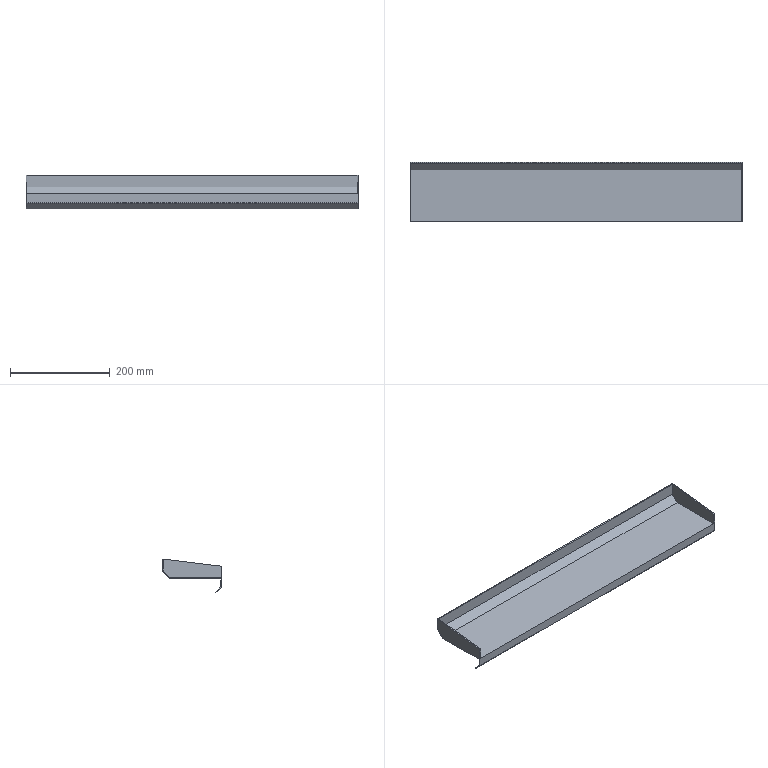Part | SolidWorks | features ICE 2, Chamfer 1, Extrusion 1, Shell 1 | 1 solid | 18 faces | box 665 x 120 x 68.021 mm | volume 255625 mm3 | plane 16 | cylinder 2 | commonest cylinder face diameters 4 x2
STEP:
#1=CARTESIAN_POINT('',(-332.5,-118.,-40.));
#2=VERTEX_POINT('',#1);
#3=CARTESIAN_POINT('',(332.5,-118.,-40.));
#4=VERTEX_POINT('',#3);
#5=CARTESIAN_POINT('',(-363.575,-118.,-40.));
#6=DIRECTION('',(1.,0.,0.));
#7=VECTOR('',#6,1000.);
#8=LINE('',#5,#7);
#9=EDGE_CURVE('',#2,#4,#8,.T.);
#10=ORIENTED_EDGE('',*,*,#9,.F.);
#11=CARTESIAN_POINT('',(-332.5,-15.,-40.));
#12=VERTEX_POINT('',#11);
#13=CARTESIAN_POINT('',(-332.5,0.,-40.));
#14=DIRECTION('',(0.,1.,0.));
#15=VECTOR('',#14,1000.);
#16=LINE('',#13,#15);
#17=EDGE_CURVE('',#2,#12,#16,.T.);
#18=ORIENTED_EDGE('',*,*,#17,.T.);
#19=CARTESIAN_POINT('',(332.5,-15.,-40.));
#20=VERTEX_POINT('',#19);
#21=CARTESIAN_POINT('',(332.5,-15.,-40.));
#22=DIRECTION('',(1.,0.,0.));
#23=VECTOR('',#22,1000.);
#24=LINE('',#21,#23);
#25=EDGE_CURVE('',#12,#20,#24,.T.);
#26=ORIENTED_EDGE('',*,*,#25,.T.);
#27=CARTESIAN_POINT('',(332.5,0.,-40.));
#28=DIRECTION('',(0.,1.,0.));
#29=VECTOR('',#28,1000.);
#30=LINE('',#27,#29);
#31=EDGE_CURVE('',#4,#20,#30,.T.);
#32=ORIENTED_EDGE('',*,*,#31,.F.);
#33=EDGE_LOOP('',(#10,#18,#26,#32));
#34=FACE_OUTER_BOUND('',#33,.T.);
#35=CARTESIAN_POINT('',(332.5,0.,-40.));
#36=DIRECTION('',(0.,0.,1.));
#37=DIRECTION('',(0.,-1.,0.));
#38=AXIS2_PLACEMENT_3D('',#35,#36,#37);
#39=PLANE('',#38);
#40=ADVANCED_FACE('',(#34),#39,.F.);
#41=CARTESIAN_POINT('',(330.5,-2.,-0.2408));
#42=VERTEX_POINT('',#41);
#43=CARTESIAN_POINT('',(330.5,-120.,-14.447));
#44=VERTEX_POINT('',#43);
#45=CARTESIAN_POINT('',(330.5,0.,0.));
#46=DIRECTION('',(0.,-0.9928,-0.1195));
#47=VECTOR('',#46,1000.);
#48=LINE('',#45,#47);
#49=EDGE_CURVE('',#42,#44,#48,.T.);
#50=ORIENTED_EDGE('',*,*,#49,.T.);
#51=CARTESIAN_POINT('',(332.5,-120.,-14.447));
#52=VERTEX_POINT('',#51);
#53=CARTESIAN_POINT('',(332.5,-120.,-14.447));
#54=DIRECTION('',(-1.,0.,0.));
#55=VECTOR('',#54,1000.);
#56=LINE('',#53,#55);
#57=EDGE_CURVE('',#52,#44,#56,.T.);
#58=ORIENTED_EDGE('',*,*,#57,.F.);
#59=CARTESIAN_POINT('',(332.5,0.,0.));
#60=VERTEX_POINT('',#59);
#61=CARTESIAN_POINT('',(332.5,-120.,-14.447));
#62=DIRECTION('',(0.,-0.9928,-0.1195));
#63=VECTOR('',#62,1000.);
#64=LINE('',#61,#63);
#65=EDGE_CURVE('',#60,#52,#64,.T.);
#66=ORIENTED_EDGE('',*,*,#65,.F.);
#67=CARTESIAN_POINT('',(-332.5,0.,0.));
#68=VERTEX_POINT('',#67);
#69=CARTESIAN_POINT('',(332.5,0.,0.));
#70=DIRECTION('',(-1.,0.,0.));
#71=VECTOR('',#70,1000.);
#72=LINE('',#69,#71);
#73=EDGE_CURVE('',#60,#68,#72,.T.);
#74=ORIENTED_EDGE('',*,*,#73,.T.);
#75=CARTESIAN_POINT('',(-332.5,-120.,-14.447));
#76=VERTEX_POINT('',#75);
#77=CARTESIAN_POINT('',(-332.5,-120.,-14.447));
#78=DIRECTION('',(0.,-0.9928,-0.1195));
#79=VECTOR('',#78,1000.);
#80=LINE('',#77,#79);
#81=EDGE_CURVE('',#68,#76,#80,.T.);
#82=ORIENTED_EDGE('',*,*,#81,.T.);
#83=CARTESIAN_POINT('',(-330.5,-120.,-14.447));
#84=VERTEX_POINT('',#83);
#85=CARTESIAN_POINT('',(332.5,-120.,-14.447));
#86=DIRECTION('',(-1.,0.,0.));
#87=VECTOR('',#86,1000.);
#88=LINE('',#85,#87);
#89=EDGE_CURVE('',#84,#76,#88,.T.);
#90=ORIENTED_EDGE('',*,*,#89,.F.);
#91=CARTESIAN_POINT('',(-330.5,-2.,-0.2408));
#92=VERTEX_POINT('',#91);
#93=CARTESIAN_POINT('',(-330.5,0.,0.));
#94=DIRECTION('',(0.,-0.9928,-0.1195));
#95=VECTOR('',#94,1000.);
#96=LINE('',#93,#95);
#97=EDGE_CURVE('',#92,#84,#96,.T.);
#98=ORIENTED_EDGE('',*,*,#97,.F.);
#99=CARTESIAN_POINT('',(332.5,-2.,-0.2408));
#100=DIRECTION('',(-1.,0.,0.));
#101=VECTOR('',#100,1000.);
#102=LINE('',#99,#101);
#103=EDGE_CURVE('',#42,#92,#102,.T.);
#104=ORIENTED_EDGE('',*,*,#103,.F.);
#105=EDGE_LOOP('',(#50,#58,#66,#74,#82,#90,#98,#104));
#106=FACE_OUTER_BOUND('',#105,.T.);
#107=CARTESIAN_POINT('',(332.5,-120.,-14.447));
#108=DIRECTION('',(0.,0.1195,-0.9928));
#109=DIRECTION('',(0.,0.9928,0.1195));
#110=AXIS2_PLACEMENT_3D('',#107,#108,#109);
#111=PLANE('',#110);
#112=ADVANCED_FACE('',(#106),#111,.F.);
#113=ORIENTED_EDGE('',*,*,#57,.T.);
#114=CARTESIAN_POINT('',(330.5,-120.,-38.));
#115=VERTEX_POINT('',#114);
#116=CARTESIAN_POINT('',(330.5,-120.,-14.206));
#117=DIRECTION('',(0.,0.,-1.));
#118=VECTOR('',#117,1000.);
#119=LINE('',#116,#118);
#120=EDGE_CURVE('',#44,#115,#119,.T.);
#121=ORIENTED_EDGE('',*,*,#120,.T.);
#122=CARTESIAN_POINT('',(-330.5,-120.,-38.));
#123=VERTEX_POINT('',#122);
#124=CARTESIAN_POINT('',(330.5,-120.,-38.));
#125=DIRECTION('',(-1.,0.,0.));
#126=VECTOR('',#125,1000.);
#127=LINE('',#124,#126);
#128=EDGE_CURVE('',#115,#123,#127,.T.);
#129=ORIENTED_EDGE('',*,*,#128,.T.);
#130=CARTESIAN_POINT('',(-330.5,-120.,-38.));
#131=DIRECTION('',(0.,0.,1.));
#132=VECTOR('',#131,1000.);
#133=LINE('',#130,#132);
#134=EDGE_CURVE('',#123,#84,#133,.T.);
#135=ORIENTED_EDGE('',*,*,#134,.T.);
#136=ORIENTED_EDGE('',*,*,#89,.T.);
#137=CARTESIAN_POINT('',(-332.5,-120.,-55.172));
#138=VERTEX_POINT('',#137);
#139=CARTESIAN_POINT('',(-332.5,-120.,-14.447));
#140=DIRECTION('',(0.,0.,-1.));
#141=VECTOR('',#140,1000.);
#142=LINE('',#139,#141);
#143=EDGE_CURVE('',#76,#138,#142,.T.);
#144=ORIENTED_EDGE('',*,*,#143,.T.);
#145=CARTESIAN_POINT('',(332.5,-120.,-55.172));
#146=VERTEX_POINT('',#145);
#147=CARTESIAN_POINT('',(-363.575,-120.,-55.172));
#148=DIRECTION('',(1.,0.,0.));
#149=VECTOR('',#148,1000.);
#150=LINE('',#147,#149);
#151=EDGE_CURVE('',#138,#146,#150,.T.);
#152=ORIENTED_EDGE('',*,*,#151,.T.);
#153=CARTESIAN_POINT('',(332.5,-120.,-14.447));
#154=DIRECTION('',(0.,0.,-1.));
#155=VECTOR('',#154,1000.);
#156=LINE('',#153,#155);
#157=EDGE_CURVE('',#52,#146,#156,.T.);
#158=ORIENTED_EDGE('',*,*,#157,.F.);
#159=EDGE_LOOP('',(#113,#121,#129,#135,#136,#144,#152,#158));
#160=FACE_OUTER_BOUND('',#159,.T.);
#161=CARTESIAN_POINT('',(332.5,-120.,-14.447));
#162=DIRECTION('',(0.,1.,0.));
#163=DIRECTION('',(0.,0.,1.));
#164=AXIS2_PLACEMENT_3D('',#161,#162,#163);
#165=PLANE('',#164);
#166=ADVANCED_FACE('',(#160),#165,.F.);
#167=CARTESIAN_POINT('',(332.5,0.,-25.));
#168=VERTEX_POINT('',#167);
#169=CARTESIAN_POINT('',(332.5,0.,0.));
#170=DIRECTION('',(0.,0.,1.));
#171=VECTOR('',#170,1000.);
#172=LINE('',#169,#171);
#173=EDGE_CURVE('',#168,#60,#172,.T.);
#174=ORIENTED_EDGE('',*,*,#173,.F.);
#175=CARTESIAN_POINT('',(-332.5,0.,-25.));
#176=VERTEX_POINT('',#175);
#177=CARTESIAN_POINT('',(332.5,0.,-25.));
#178=DIRECTION('',(-1.,0.,0.));
#179=VECTOR('',#178,1000.);
#180=LINE('',#177,#179);
#181=EDGE_CURVE('',#168,#176,#180,.T.);
#182=ORIENTED_EDGE('',*,*,#181,.T.);
#183=CARTESIAN_POINT('',(-332.5,0.,0.));
#184=DIRECTION('',(0.,0.,1.));
#185=VECTOR('',#184,1000.);
#186=LINE('',#183,#185);
#187=EDGE_CURVE('',#176,#68,#186,.T.);
#188=ORIENTED_EDGE('',*,*,#187,.T.);
#189=ORIENTED_EDGE('',*,*,#73,.F.);
#190=EDGE_LOOP('',(#174,#182,#188,#189));
#191=FACE_OUTER_BOUND('',#190,.T.);
#192=CARTESIAN_POINT('',(332.5,0.,0.));
#193=DIRECTION('',(0.,-1.,0.));
#194=DIRECTION('',(0.,0.,-1.));
#195=AXIS2_PLACEMENT_3D('',#192,#193,#194);
#196=PLANE('',#195);
#197=ADVANCED_FACE('',(#191),#196,.F.);
#198=ORIENTED_EDGE('',*,*,#157,.T.);
#199=CARTESIAN_POINT('',(332.5,-119.414,-56.586));
#200=VERTEX_POINT('',#199);
#201=CARTESIAN_POINT('',(332.5,-118.,-55.172));
#202=DIRECTION('',(1.,0.,0.));
#203=DIRECTION('',(0.,0.,1.));
#204=AXIS2_PLACEMENT_3D('',#201,#202,#203);
#205=CIRCLE('',#204,2.);
#206=EDGE_CURVE('',#146,#200,#205,.T.);
#207=ORIENTED_EDGE('',*,*,#206,.T.);
#208=CARTESIAN_POINT('',(332.5,-107.979,-68.021));
#209=VERTEX_POINT('',#208);
#210=CARTESIAN_POINT('',(332.5,-119.414,-56.586));
#211=DIRECTION('',(0.,0.7071,-0.7071));
#212=VECTOR('',#211,1000.);
#213=LINE('',#210,#212);
#214=EDGE_CURVE('',#200,#209,#213,.T.);
#215=ORIENTED_EDGE('',*,*,#214,.T.);
#216=CARTESIAN_POINT('',(332.5,-106.565,-66.607));
#217=VERTEX_POINT('',#216);
#218=CARTESIAN_POINT('',(332.5,-107.979,-68.021));
#219=DIRECTION('',(0.,0.7071,0.7071));
#220=VECTOR('',#219,1000.);
#221=LINE('',#218,#220);
#222=EDGE_CURVE('',#209,#217,#221,.T.);
#223=ORIENTED_EDGE('',*,*,#222,.T.);
#224=CARTESIAN_POINT('',(332.5,-117.414,-55.757));
#225=VERTEX_POINT('',#224);
#226=CARTESIAN_POINT('',(332.5,-106.565,-66.607));
#227=DIRECTION('',(0.,-0.7071,0.7071));
#228=VECTOR('',#227,1000.);
#229=LINE('',#226,#228);
#230=EDGE_CURVE('',#217,#225,#229,.T.);
#231=ORIENTED_EDGE('',*,*,#230,.T.);
#232=CARTESIAN_POINT('',(332.5,-118.,-54.343));
#233=VERTEX_POINT('',#232);
#234=CARTESIAN_POINT('',(332.5,-116.,-54.343));
#235=DIRECTION('',(-1.,0.,0.));
#236=DIRECTION('',(0.,0.,1.));
#237=AXIS2_PLACEMENT_3D('',#234,#235,#236);
#238=CIRCLE('',#237,2.);
#239=EDGE_CURVE('',#225,#233,#238,.T.);
#240=ORIENTED_EDGE('',*,*,#239,.T.);
#241=CARTESIAN_POINT('',(332.5,-118.,-54.343));
#242=DIRECTION('',(0.,0.,1.));
#243=VECTOR('',#242,1000.);
#244=LINE('',#241,#243);
#245=EDGE_CURVE('',#233,#4,#244,.T.);
#246=ORIENTED_EDGE('',*,*,#245,.T.);
#247=ORIENTED_EDGE('',*,*,#31,.T.);
#248=CARTESIAN_POINT('',(332.5,0.,-25.));
#249=DIRECTION('',(0.,0.7071,0.7071));
#250=VECTOR('',#249,1000.);
#251=LINE('',#248,#250);
#252=EDGE_CURVE('',#20,#168,#251,.T.);
#253=ORIENTED_EDGE('',*,*,#252,.T.);
#254=ORIENTED_EDGE('',*,*,#173,.T.);
#255=ORIENTED_EDGE('',*,*,#65,.T.);
#256=EDGE_LOOP('',(#198,#207,#215,#223,#231,#240,#246,#247,#253,#254,#255));
#257=FACE_OUTER_BOUND('',#256,.T.);
#258=CARTESIAN_POINT('',(332.5,0.,0.));
#259=DIRECTION('',(-1.,0.,0.));
#260=DIRECTION('',(0.,0.,1.));
#261=AXIS2_PLACEMENT_3D('',#258,#259,#260);
#262=PLANE('',#261);
#263=ADVANCED_FACE('',(#257),#262,.F.);
#264=ORIENTED_EDGE('',*,*,#187,.F.);
#265=CARTESIAN_POINT('',(-332.5,12.5,-12.5));
#266=DIRECTION('',(0.,-0.7071,-0.7071));
#267=VECTOR('',#266,1000.);
#268=LINE('',#265,#267);
#269=EDGE_CURVE('',#176,#12,#268,.T.);
#270=ORIENTED_EDGE('',*,*,#269,.T.);
#271=ORIENTED_EDGE('',*,*,#17,.F.);
#272=CARTESIAN_POINT('',(-332.5,-118.,-54.343));
#273=VERTEX_POINT('',#272);
#274=CARTESIAN_POINT('',(-332.5,-118.,-54.343));
#275=DIRECTION('',(0.,0.,1.));
#276=VECTOR('',#275,1000.);
#277=LINE('',#274,#276);
#278=EDGE_CURVE('',#273,#2,#277,.T.);
#279=ORIENTED_EDGE('',*,*,#278,.F.);
#280=CARTESIAN_POINT('',(-332.5,-117.414,-55.757));
#281=VERTEX_POINT('',#280);
#282=CARTESIAN_POINT('',(-332.5,-116.,-54.343));
#283=DIRECTION('',(-1.,0.,0.));
#284=DIRECTION('',(0.,0.,1.));
#285=AXIS2_PLACEMENT_3D('',#282,#283,#284);
#286=CIRCLE('',#285,2.);
#287=EDGE_CURVE('',#281,#273,#286,.T.);
#288=ORIENTED_EDGE('',*,*,#287,.F.);
#289=CARTESIAN_POINT('',(-332.5,-106.565,-66.607));
#290=VERTEX_POINT('',#289);
#291=CARTESIAN_POINT('',(-332.5,-106.565,-66.607));
#292=DIRECTION('',(0.,-0.7071,0.7071));
#293=VECTOR('',#292,1000.);
#294=LINE('',#291,#293);
#295=EDGE_CURVE('',#290,#281,#294,.T.);
#296=ORIENTED_EDGE('',*,*,#295,.F.);
#297=CARTESIAN_POINT('',(-332.5,-107.979,-68.021));
#298=VERTEX_POINT('',#297);
#299=CARTESIAN_POINT('',(-332.5,-107.979,-68.021));
#300=DIRECTION('',(0.,0.7071,0.7071));
#301=VECTOR('',#300,1000.);
#302=LINE('',#299,#301);
#303=EDGE_CURVE('',#298,#290,#302,.T.);
#304=ORIENTED_EDGE('',*,*,#303,.F.);
#305=CARTESIAN_POINT('',(-332.5,-119.414,-56.586));
#306=VERTEX_POINT('',#305);
#307=CARTESIAN_POINT('',(-332.5,-119.414,-56.586));
#308=DIRECTION('',(0.,0.7071,-0.7071));
#309=VECTOR('',#308,1000.);
#310=LINE('',#307,#309);
#311=EDGE_CURVE('',#306,#298,#310,.T.);
#312=ORIENTED_EDGE('',*,*,#311,.F.);
#313=CARTESIAN_POINT('',(-332.5,-118.,-55.172));
#314=DIRECTION('',(1.,0.,0.));
#315=DIRECTION('',(0.,0.,1.));
#316=AXIS2_PLACEMENT_3D('',#313,#314,#315);
#317=CIRCLE('',#316,2.);
#318=EDGE_CURVE('',#138,#306,#317,.T.);
#319=ORIENTED_EDGE('',*,*,#318,.F.);
#320=ORIENTED_EDGE('',*,*,#143,.F.);
#321=ORIENTED_EDGE('',*,*,#81,.F.);
#322=EDGE_LOOP('',(#264,#270,#271,#279,#288,#296,#304,#312,#319,#320,#321));
#323=FACE_OUTER_BOUND('',#322,.T.);
#324=CARTESIAN_POINT('',(-332.5,0.,0.));
#325=DIRECTION('',(-1.,0.,0.));
#326=DIRECTION('',(0.,0.,1.));
#327=AXIS2_PLACEMENT_3D('',#324,#325,#326);
#328=PLANE('',#327);
#329=ADVANCED_FACE('',(#323),#328,.T.);
#330=ORIENTED_EDGE('',*,*,#252,.F.);
#331=ORIENTED_EDGE('',*,*,#25,.F.);
#332=ORIENTED_EDGE('',*,*,#269,.F.);
#333=ORIENTED_EDGE('',*,*,#181,.F.);
#334=EDGE_LOOP('',(#330,#331,#332,#333));
#335=FACE_OUTER_BOUND('',#334,.T.);
#336=CARTESIAN_POINT('',(332.5,0.,-25.));
#337=DIRECTION('',(0.,-0.7071,0.7071));
#338=DIRECTION('',(-1.,0.,0.));
#339=AXIS2_PLACEMENT_3D('',#336,#337,#338);
#340=PLANE('',#339);
#341=ADVANCED_FACE('',(#335),#340,.F.);
#342=CARTESIAN_POINT('',(-330.5,-15.828,-38.));
#343=VERTEX_POINT('',#342);
#344=CARTESIAN_POINT('',(-330.5,0.,-38.));
#345=DIRECTION('',(0.,1.,0.));
#346=VECTOR('',#345,1000.);
#347=LINE('',#344,#346);
#348=EDGE_CURVE('',#123,#343,#347,.T.);
#349=ORIENTED_EDGE('',*,*,#348,.F.);
#350=ORIENTED_EDGE('',*,*,#128,.F.);
#351=CARTESIAN_POINT('',(330.5,-15.828,-38.));
#352=VERTEX_POINT('',#351);
#353=CARTESIAN_POINT('',(330.5,0.,-38.));
#354=DIRECTION('',(0.,1.,0.));
#355=VECTOR('',#354,1000.);
#356=LINE('',#353,#355);
#357=EDGE_CURVE('',#115,#352,#356,.T.);
#358=ORIENTED_EDGE('',*,*,#357,.T.);
#359=CARTESIAN_POINT('',(332.5,-15.828,-38.));
#360=DIRECTION('',(1.,0.,0.));
#361=VECTOR('',#360,1000.);
#362=LINE('',#359,#361);
#363=EDGE_CURVE('',#343,#352,#362,.T.);
#364=ORIENTED_EDGE('',*,*,#363,.F.);
#365=EDGE_LOOP('',(#349,#350,#358,#364));
#366=FACE_OUTER_BOUND('',#365,.T.);
#367=CARTESIAN_POINT('',(332.5,0.,-38.));
#368=DIRECTION('',(0.,0.,1.));
#369=DIRECTION('',(0.,-1.,0.));
#370=AXIS2_PLACEMENT_3D('',#367,#368,#369);
#371=PLANE('',#370);
#372=ADVANCED_FACE('',(#366),#371,.T.);
#373=CARTESIAN_POINT('',(330.5,-2.,-24.172));
#374=VERTEX_POINT('',#373);
#375=CARTESIAN_POINT('',(330.5,-2.,0.));
#376=DIRECTION('',(0.,0.,1.));
#377=VECTOR('',#376,1000.);
#378=LINE('',#375,#377);
#379=EDGE_CURVE('',#374,#42,#378,.T.);
#380=ORIENTED_EDGE('',*,*,#379,.T.);
#381=ORIENTED_EDGE('',*,*,#103,.T.);
#382=CARTESIAN_POINT('',(-330.5,-2.,-24.172));
#383=VERTEX_POINT('',#382);
#384=CARTESIAN_POINT('',(-330.5,-2.,0.));
#385=DIRECTION('',(0.,0.,1.));
#386=VECTOR('',#385,1000.);
#387=LINE('',#384,#386);
#388=EDGE_CURVE('',#383,#92,#387,.T.);
#389=ORIENTED_EDGE('',*,*,#388,.F.);
#390=CARTESIAN_POINT('',(332.5,-2.,-24.172));
#391=DIRECTION('',(-1.,0.,0.));
#392=VECTOR('',#391,1000.);
#393=LINE('',#390,#392);
#394=EDGE_CURVE('',#374,#383,#393,.T.);
#395=ORIENTED_EDGE('',*,*,#394,.F.);
#396=EDGE_LOOP('',(#380,#381,#389,#395));
#397=FACE_OUTER_BOUND('',#396,.T.);
#398=CARTESIAN_POINT('',(332.5,-2.,0.));
#399=DIRECTION('',(0.,-1.,0.));
#400=DIRECTION('',(0.,0.,-1.));
#401=AXIS2_PLACEMENT_3D('',#398,#399,#400);
#402=PLANE('',#401);
#403=ADVANCED_FACE('',(#397),#402,.T.);
#404=ORIENTED_EDGE('',*,*,#357,.F.);
#405=ORIENTED_EDGE('',*,*,#120,.F.);
#406=ORIENTED_EDGE('',*,*,#49,.F.);
#407=ORIENTED_EDGE('',*,*,#379,.F.);
#408=CARTESIAN_POINT('',(330.5,-1.414,-23.586));
#409=DIRECTION('',(0.,0.7071,0.7071));
#410=VECTOR('',#409,1000.);
#411=LINE('',#408,#410);
#412=EDGE_CURVE('',#352,#374,#411,.T.);
#413=ORIENTED_EDGE('',*,*,#412,.F.);
#414=EDGE_LOOP('',(#404,#405,#406,#407,#413));
#415=FACE_OUTER_BOUND('',#414,.T.);
#416=CARTESIAN_POINT('',(330.5,0.,0.));
#417=DIRECTION('',(-1.,0.,0.));
#418=DIRECTION('',(0.,0.,1.));
#419=AXIS2_PLACEMENT_3D('',#416,#417,#418);
#420=PLANE('',#419);
#421=ADVANCED_FACE('',(#415),#420,.T.);
#422=ORIENTED_EDGE('',*,*,#388,.T.);
#423=ORIENTED_EDGE('',*,*,#97,.T.);
#424=ORIENTED_EDGE('',*,*,#134,.F.);
#425=ORIENTED_EDGE('',*,*,#348,.T.);
#426=CARTESIAN_POINT('',(-330.5,11.086,-11.086));
#427=DIRECTION('',(0.,-0.7071,-0.7071));
#428=VECTOR('',#427,1000.);
#429=LINE('',#426,#428);
#430=EDGE_CURVE('',#383,#343,#429,.T.);
#431=ORIENTED_EDGE('',*,*,#430,.F.);
#432=EDGE_LOOP('',(#422,#423,#424,#425,#431));
#433=FACE_OUTER_BOUND('',#432,.T.);
#434=CARTESIAN_POINT('',(-330.5,0.,0.));
#435=DIRECTION('',(-1.,0.,0.));
#436=DIRECTION('',(0.,0.,1.));
#437=AXIS2_PLACEMENT_3D('',#434,#435,#436);
#438=PLANE('',#437);
#439=ADVANCED_FACE('',(#433),#438,.F.);
#440=ORIENTED_EDGE('',*,*,#412,.T.);
#441=ORIENTED_EDGE('',*,*,#394,.T.);
#442=ORIENTED_EDGE('',*,*,#430,.T.);
#443=ORIENTED_EDGE('',*,*,#363,.T.);
#444=EDGE_LOOP('',(#440,#441,#442,#443));
#445=FACE_OUTER_BOUND('',#444,.T.);
#446=CARTESIAN_POINT('',(332.5,-1.414,-23.586));
#447=DIRECTION('',(0.,-0.7071,0.7071));
#448=DIRECTION('',(-1.,0.,0.));
#449=AXIS2_PLACEMENT_3D('',#446,#447,#448);
#450=PLANE('',#449);
#451=ADVANCED_FACE('',(#445),#450,.T.);
#452=ORIENTED_EDGE('',*,*,#151,.F.);
#453=ORIENTED_EDGE('',*,*,#318,.T.);
#454=CARTESIAN_POINT('',(-363.575,-119.414,-56.586));
#455=DIRECTION('',(1.,0.,0.));
#456=VECTOR('',#455,1000.);
#457=LINE('',#454,#456);
#458=EDGE_CURVE('',#306,#200,#457,.T.);
#459=ORIENTED_EDGE('',*,*,#458,.T.);
#460=ORIENTED_EDGE('',*,*,#206,.F.);
#461=EDGE_LOOP('',(#452,#453,#459,#460));
#462=FACE_OUTER_BOUND('',#461,.T.);
#463=CARTESIAN_POINT('',(-363.575,-118.,-55.172));
#464=DIRECTION('',(1.,0.,0.));
#465=DIRECTION('',(0.,0.,-1.));
#466=AXIS2_PLACEMENT_3D('',#463,#464,#465);
#467=CYLINDRICAL_SURFACE('',#466,2.);
#468=ADVANCED_FACE('',(#462),#467,.T.);
#469=ORIENTED_EDGE('',*,*,#458,.F.);
#470=ORIENTED_EDGE('',*,*,#311,.T.);
#471=CARTESIAN_POINT('',(-363.575,-107.979,-68.021));
#472=DIRECTION('',(1.,0.,0.));
#473=VECTOR('',#472,1000.);
#474=LINE('',#471,#473);
#475=EDGE_CURVE('',#298,#209,#474,.T.);
#476=ORIENTED_EDGE('',*,*,#475,.T.);
#477=ORIENTED_EDGE('',*,*,#214,.F.);
#478=EDGE_LOOP('',(#469,#470,#476,#477));
#479=FACE_OUTER_BOUND('',#478,.T.);
#480=CARTESIAN_POINT('',(-363.575,-119.414,-56.586));
#481=DIRECTION('',(0.,-0.7071,-0.7071));
#482=DIRECTION('',(0.,0.7071,-0.7071));
#483=AXIS2_PLACEMENT_3D('',#480,#481,#482);
#484=PLANE('',#483);
#485=ADVANCED_FACE('',(#479),#484,.T.);
#486=ORIENTED_EDGE('',*,*,#475,.F.);
#487=ORIENTED_EDGE('',*,*,#303,.T.);
#488=CARTESIAN_POINT('',(-363.575,-106.565,-66.607));
#489=DIRECTION('',(1.,0.,0.));
#490=VECTOR('',#489,1000.);
#491=LINE('',#488,#490);
#492=EDGE_CURVE('',#290,#217,#491,.T.);
#493=ORIENTED_EDGE('',*,*,#492,.T.);
#494=ORIENTED_EDGE('',*,*,#222,.F.);
#495=EDGE_LOOP('',(#486,#487,#493,#494));
#496=FACE_OUTER_BOUND('',#495,.T.);
#497=CARTESIAN_POINT('',(-363.575,-107.979,-68.021));
#498=DIRECTION('',(0.,0.7071,-0.7071));
#499=DIRECTION('',(0.,0.7071,0.7071));
#500=AXIS2_PLACEMENT_3D('',#497,#498,#499);
#501=PLANE('',#500);
#502=ADVANCED_FACE('',(#496),#501,.T.);
#503=ORIENTED_EDGE('',*,*,#492,.F.);
#504=ORIENTED_EDGE('',*,*,#295,.T.);
#505=CARTESIAN_POINT('',(-363.575,-117.414,-55.757));
#506=DIRECTION('',(1.,0.,0.));
#507=VECTOR('',#506,1000.);
#508=LINE('',#505,#507);
#509=EDGE_CURVE('',#281,#225,#508,.T.);
#510=ORIENTED_EDGE('',*,*,#509,.T.);
#511=ORIENTED_EDGE('',*,*,#230,.F.);
#512=EDGE_LOOP('',(#503,#504,#510,#511));
#513=FACE_OUTER_BOUND('',#512,.T.);
#514=CARTESIAN_POINT('',(-363.575,-106.565,-66.607));
#515=DIRECTION('',(0.,0.7071,0.7071));
#516=DIRECTION('',(0.,-0.7071,0.7071));
#517=AXIS2_PLACEMENT_3D('',#514,#515,#516);
#518=PLANE('',#517);
#519=ADVANCED_FACE('',(#513),#518,.T.);
#520=ORIENTED_EDGE('',*,*,#509,.F.);
#521=ORIENTED_EDGE('',*,*,#287,.T.);
#522=CARTESIAN_POINT('',(-363.575,-118.,-54.343));
#523=DIRECTION('',(1.,0.,0.));
#524=VECTOR('',#523,1000.);
#525=LINE('',#522,#524);
#526=EDGE_CURVE('',#273,#233,#525,.T.);
#527=ORIENTED_EDGE('',*,*,#526,.T.);
#528=ORIENTED_EDGE('',*,*,#239,.F.);
#529=EDGE_LOOP('',(#520,#521,#527,#528));
#530=FACE_OUTER_BOUND('',#529,.T.);
#531=CARTESIAN_POINT('',(-363.575,-116.,-54.343));
#532=DIRECTION('',(1.,0.,0.));
#533=DIRECTION('',(0.,0.,-1.));
#534=AXIS2_PLACEMENT_3D('',#531,#532,#533);
#535=CYLINDRICAL_SURFACE('',#534,2.);
#536=ADVANCED_FACE('',(#530),#535,.F.);
#537=ORIENTED_EDGE('',*,*,#526,.F.);
#538=ORIENTED_EDGE('',*,*,#278,.T.);
#539=ORIENTED_EDGE('',*,*,#9,.T.);
#540=ORIENTED_EDGE('',*,*,#245,.F.);
#541=EDGE_LOOP('',(#537,#538,#539,#540));
#542=FACE_OUTER_BOUND('',#541,.T.);
#543=CARTESIAN_POINT('',(-363.575,-118.,-54.343));
#544=DIRECTION('',(0.,1.,0.));
#545=DIRECTION('',(0.,0.,1.));
#546=AXIS2_PLACEMENT_3D('',#543,#544,#545);
#547=PLANE('',#546);
#548=ADVANCED_FACE('',(#542),#547,.T.);
#549=CLOSED_SHELL('',(#40,#112,#166,#197,#263,#329,#341,#372,#403,#421,#439,#451,#468,#485,#502,#519,#536,#548));
#550=MANIFOLD_SOLID_BREP('',#549);
#551=CARTESIAN_POINT('',(0.,0.,0.));
#552=DIRECTION('',(0.,0.,1.));
#553=DIRECTION('',(1.,0.,0.));
#554=AXIS2_PLACEMENT_3D('',#551,#552,#553);
#555=(LENGTH_UNIT()NAMED_UNIT(*)SI_UNIT(.MILLI.,.METRE.));
#556=UNCERTAINTY_MEASURE_WITH_UNIT(LENGTH_MEASURE(0.00001),#555,'','');
#557=(NAMED_UNIT(*)PLANE_ANGLE_UNIT()SI_UNIT($,.RADIAN.));
#558=(NAMED_UNIT(*)SI_UNIT($,.STERADIAN.)SOLID_ANGLE_UNIT());
#559=(GEOMETRIC_REPRESENTATION_CONTEXT(3)GLOBAL_UNCERTAINTY_ASSIGNED_CONTEXT((#556))GLOBAL_UNIT_ASSIGNED_CONTEXT((#555,#557,#558))REPRESENTATION_CONTEXT('',''));
#560=ADVANCED_BREP_SHAPE_REPRESENTATION('',(#550,#554),#559);